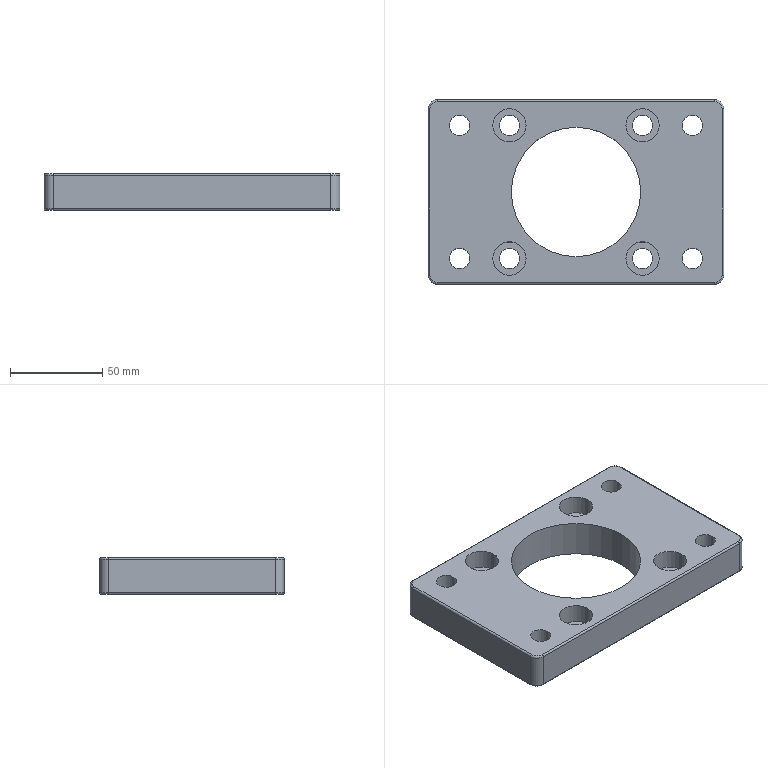Part | SolidWorks | features Fillet 2, HoleWzd 2, Extrusion 1 | 1 solid | 68 faces | box 160 x 100 x 20 mm | volume 213466 mm3 | cylinder 46 | plane 14 | torus 8 | commonest cylinder face diameters 11 x16 18 x16 2 x8 10 x4 70 x2